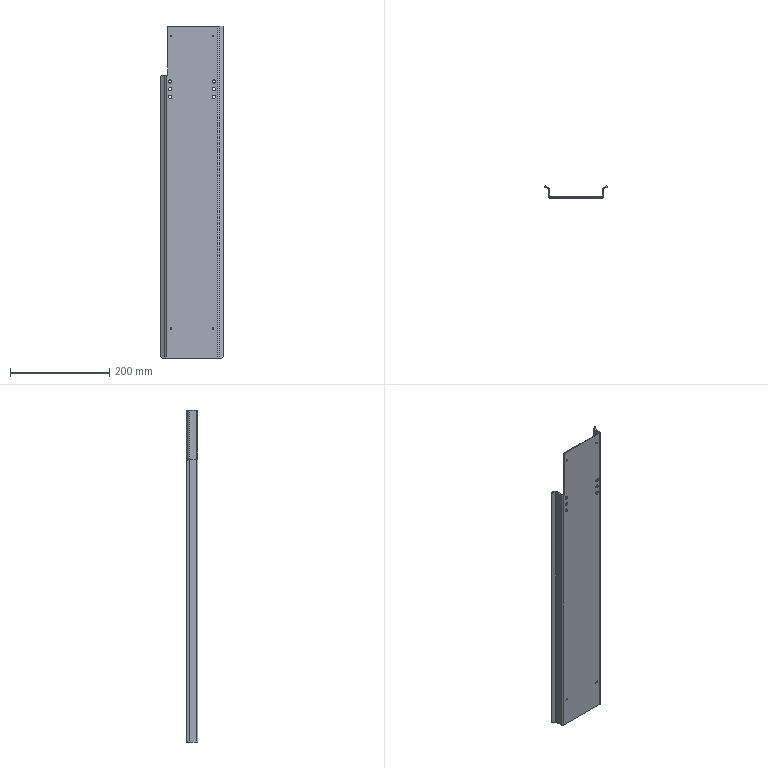Part | STEP file | 1 solid | 72 faces | box 125.321 x 23.845 x 670 mm | volume 206650 mm3 | cylinder 33 | plane 31 | cone 8 | commonest cylinder face diameters 6.6 x12 6 x9 3.4 x8 2 x4